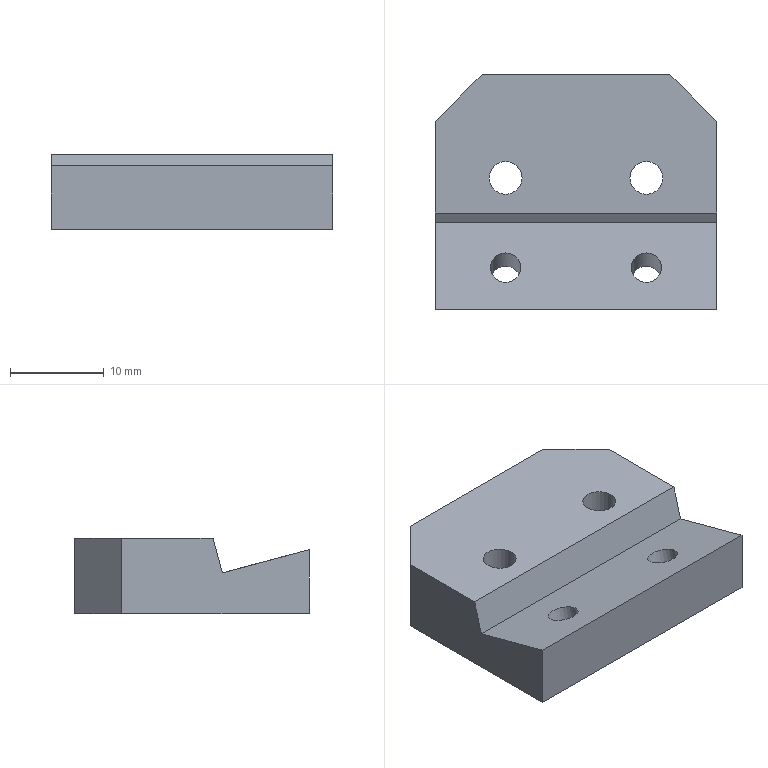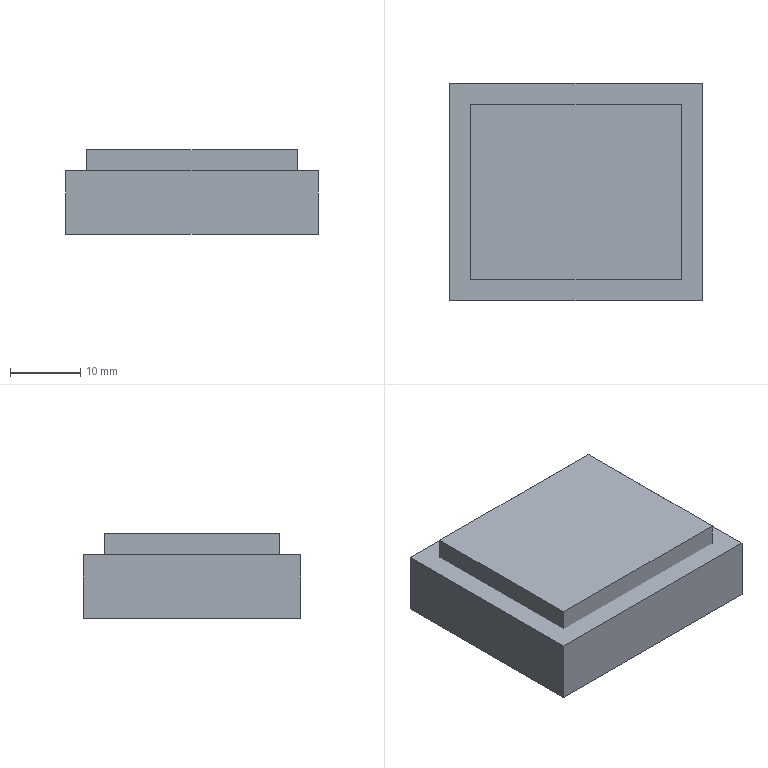CAM job | NX | 3+2 milling, drilling | part box 30 x 25 x 8 mm | stock box 36 x 31 x 12 mm
Tools:
number,name,description,diameter,corner_radius,flute_length,length,flutes
1,D63,Milling Tool-5 Parameters,63.0,0.0,50.0,75.0,2
9,D6A45,Milling Tool-5 Parameters,6.0,0.0,3.0,3.0,2
12,3.5ZT,Drilling Tool,3.5,0.0,35.0,50.0,2
2,D10,Milling Tool-5 Parameters,10.0,0.0,50.0,75.0,2
4,D6,Milling Tool-5 Parameters,6.0,0.0,50.0,75.0,2
16,D3R0.5,Milling Tool-5 Parameters,3.0,0.5,50.0,75.0,2
8,D2,Milling Tool-5 Parameters,2.0,0.0,50.0,75.0,2
Operations:
program,operation,operation_type,tool,method,geometry_group,spindle_rpm,surface_speed,feed_per_tooth,feed_cut,feed_plunge,cut_length_mm,path_length_mm,cut_time_min,machine_time_min
1-35-30-12毛胚-桥板,FLOOR_WALL,VolumeBased25DMillingOperation,D63,METHOD,A,6500.0,0.0,0.0,1250.0,100.0,106.0,160.0,0.0848,0.0902
1-35-30-12毛胚-桥板,DRILLING,Operation,D6A45,METHOD,A,4000.0,75.0,0.0312,250.0,0.0,8.0,94.297,0.032,0.0406
1-35-30-12毛胚-桥板,DRILLING_COPY_1,Operation,3.5ZT,METHOD,A,2000.0,20.0,0.05,200.0,0.0,27.103,132.503,0.1355,0.1461
1-35-30-12毛胚-桥板,ADAPTIVE_MILLING,CavityMilling,D10,METHOD,A,7000.0,219.0,0.1429,2000.0,1000.0,736.99,806.99,0.37,0.377
1-35-30-12毛胚-桥板,ZLEVEL_PROFILE_COPY_COPY_1_COPY_COPY_COPY,ZLevelMilling,D10,METHOD,A,7000.0,65.0,0.1429,2000.0,1000.0,353.241,517.776,0.1811,0.1975
1-35-30-12毛胚-桥板,ZLEVEL_PROFILE_COPY_COPY_1_COPY,ZLevelMilling,D6,METHOD,A,6500.0,326.0,0.0769,1000.0,1000.0,129.592,202.592,0.1296,0.1369
1-35-30-12毛胚-桥板,ZLEVEL_PROFILE_COPY_COPY_1_COPY_COPY,ZLevelMilling,D3R0.5,METHOD,A,7000.0,65.0,0.1429,2000.0,1000.0,6139.986,6295.648,3.072,3.088
1-35-30-12毛胚-桥板,ZLEVEL_PROFILE_COPY_1_COPY_COPY_COPY_COPY,ZLevelMilling,D6A45,METHOD,A,7000.0,131.0,0.0714,1000.0,1000.0,106.208,316.596,0.1062,0.1272
2-35-30-12毛胚-桥板,ZLEVEL_PROFILE_COPY_COPY_1_COPY_COPY_1,ZLevelMilling,D10,METHOD,B,6500.0,326.0,0.0769,1000.0,1000.0,49.046,106.046,0.049,0.0547
2-35-30-12毛胚-桥板,HOLE_MILLING,CylinderMilling,D2,METHOD,B,9500.0,59.0,0.0526,1000.0,100.0,578.153,723.665,0.5782,0.5927
2-35-30-12毛胚-桥板,ZLEVEL_PROFILE_COPY_1_COPY_COPY_COPY_COPY_COPY,ZLevelMilling,D6A45,METHOD,B,7000.0,131.0,0.0714,1000.0,1000.0,61.037,284.731,0.061,0.0834
3-35-30-12毛胚,FLOOR_WALL_COPY,VolumeBased25DMillingOperation,D63,METHOD,C,6500.0,0.0,0.0,1250.0,100.0,420.0,921.001,0.336,0.3861
3-35-30-12毛胚,ZLEVEL_PROFILE_COPY_1_COPY_COPY_COPY_COPY_COPY_1,ZLevelMilling,D6A45,METHOD,C,7000.0,131.0,0.0714,1000.0,1000.0,126.722,345.317,0.1267,0.1486